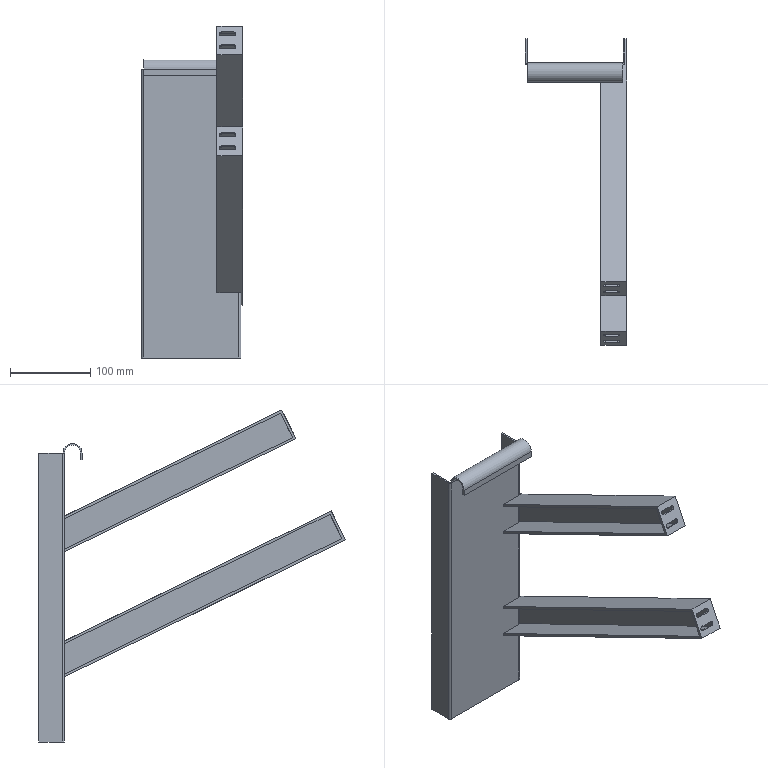Part | STEP file | 11-FG-B08611 | 1 solid | 70 faces | box 126 x 381.8 x 413.682 mm | volume 331589 mm3 | plane 56 | cylinder 14 | commonest cylinder face diameters 5.5 x8 1.473 x2 5.473 x2 20 x1 24 x1